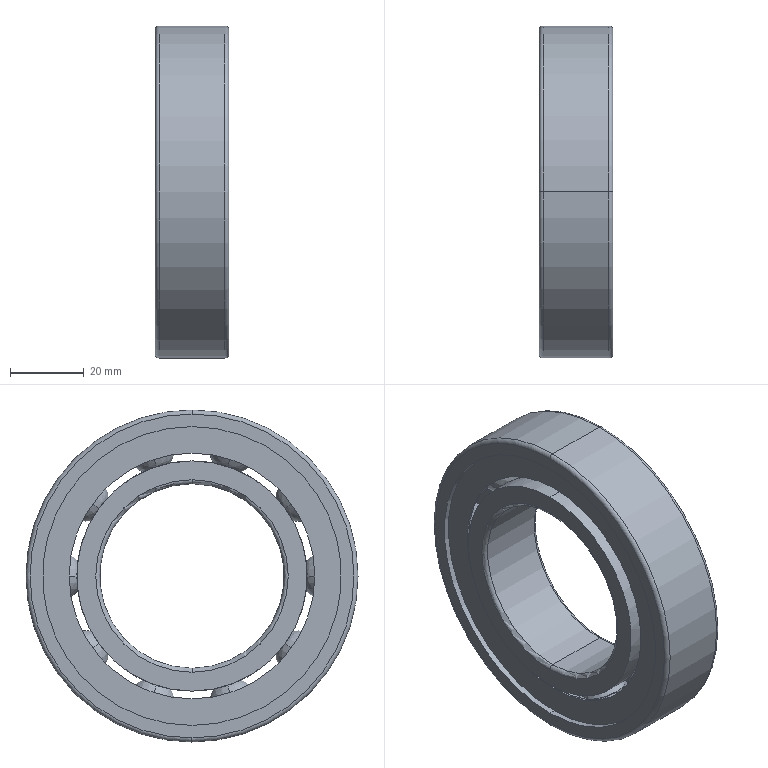Part | SolidWorks | features Revolution 6, CirPattern 2, RevCut 2, MirrorPattern 1 | 1 solid | 173 faces | box 20 x 90 x 90 mm | volume 55631 mm3 | sphere 80 | torus 41 | plane 28 | cylinder 24 | commonest cylinder face diameters 81 x8 62.4 x4 66.591 x4 50 x2 68.208 x2 75.192 x2